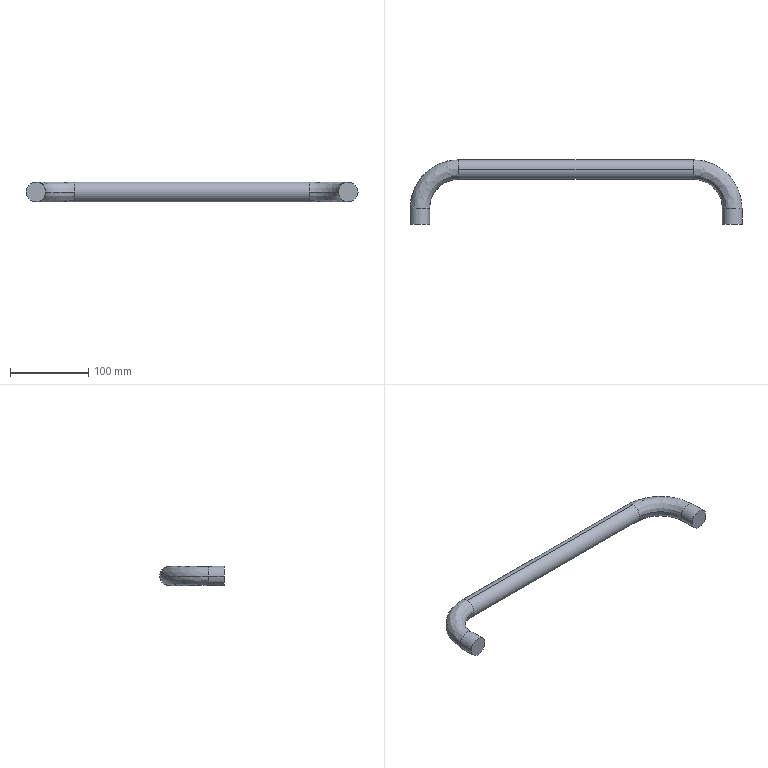Part | STEP file | 921270223 | 1 solid | 12 faces | box 425 x 82.5 x 25 mm | volume 244003 mm3 | cylinder 6 | spline 4 | plane 2 | commonest cylinder face diameters 25 x6
STEP:
#1=CARTESIAN_POINT('',(350.,82.5,0.));
#2=VERTEX_POINT('',#1);
#3=CARTESIAN_POINT('',(350.,70.,-12.5));
#4=VERTEX_POINT('',#3);
#5=CARTESIAN_POINT('',(350.,70.,0.));
#6=DIRECTION('',(-1.,0.,0.));
#7=DIRECTION('',(0.,0.,1.));
#8=AXIS2_PLACEMENT_3D('',#5,#6,#7);
#9=CIRCLE('',#8,12.5);
#10=EDGE_CURVE('',#2,#4,#9,.T.);
#11=ORIENTED_EDGE('',*,*,#10,.T.);
#12=CARTESIAN_POINT('',(50.,70.,-12.5));
#13=VERTEX_POINT('',#12);
#14=CARTESIAN_POINT('',(350.,70.,-12.5));
#15=DIRECTION('',(-1.,0.,0.));
#16=VECTOR('',#15,1000.);
#17=LINE('',#14,#16);
#18=EDGE_CURVE('',#4,#13,#17,.T.);
#19=ORIENTED_EDGE('',*,*,#18,.T.);
#20=CARTESIAN_POINT('',(50.,82.5,0.));
#21=VERTEX_POINT('',#20);
#22=CARTESIAN_POINT('',(50.,70.,0.));
#23=DIRECTION('',(1.,0.,0.));
#24=DIRECTION('',(0.,0.,1.));
#25=AXIS2_PLACEMENT_3D('',#22,#23,#24);
#26=CIRCLE('',#25,12.5);
#27=EDGE_CURVE('',#13,#21,#26,.T.);
#28=ORIENTED_EDGE('',*,*,#27,.T.);
#29=CARTESIAN_POINT('',(50.,70.,12.5));
#30=VERTEX_POINT('',#29);
#31=CARTESIAN_POINT('',(50.,70.,0.));
#32=DIRECTION('',(1.,0.,0.));
#33=DIRECTION('',(0.,0.,1.));
#34=AXIS2_PLACEMENT_3D('',#31,#32,#33);
#35=CIRCLE('',#34,12.5);
#36=EDGE_CURVE('',#21,#30,#35,.T.);
#37=ORIENTED_EDGE('',*,*,#36,.T.);
#38=CARTESIAN_POINT('',(350.,70.,12.5));
#39=VERTEX_POINT('',#38);
#40=CARTESIAN_POINT('',(350.,70.,12.5));
#41=DIRECTION('',(-1.,0.,0.));
#42=VECTOR('',#41,1000.);
#43=LINE('',#40,#42);
#44=EDGE_CURVE('',#39,#30,#43,.T.);
#45=ORIENTED_EDGE('',*,*,#44,.F.);
#46=CARTESIAN_POINT('',(350.,70.,0.));
#47=DIRECTION('',(-1.,0.,0.));
#48=DIRECTION('',(0.,0.,1.));
#49=AXIS2_PLACEMENT_3D('',#46,#47,#48);
#50=CIRCLE('',#49,12.5);
#51=EDGE_CURVE('',#39,#2,#50,.T.);
#52=ORIENTED_EDGE('',*,*,#51,.T.);
#53=EDGE_LOOP('',(#11,#19,#28,#37,#45,#52));
#54=FACE_OUTER_BOUND('',#53,.T.);
#55=CARTESIAN_POINT('',(350.,70.,0.));
#56=DIRECTION('',(-1.,0.,0.));
#57=DIRECTION('',(0.,0.,1.));
#58=AXIS2_PLACEMENT_3D('',#55,#56,#57);
#59=CYLINDRICAL_SURFACE('',#58,12.5);
#60=ADVANCED_FACE('',(#54),#59,.T.);
#61=CARTESIAN_POINT('',(50.,57.5,0.));
#62=VERTEX_POINT('',#61);
#63=CARTESIAN_POINT('',(50.,70.,0.));
#64=DIRECTION('',(1.,0.,0.));
#65=DIRECTION('',(0.,0.,1.));
#66=AXIS2_PLACEMENT_3D('',#63,#64,#65);
#67=CIRCLE('',#66,12.5);
#68=EDGE_CURVE('',#62,#13,#67,.T.);
#69=ORIENTED_EDGE('',*,*,#68,.F.);
#70=CARTESIAN_POINT('',(12.5,20.,0.));
#71=VERTEX_POINT('',#70);
#72=CARTESIAN_POINT('',(50.,20.,0.));
#73=DIRECTION('',(0.,0.,1.));
#74=DIRECTION('',(1.,0.,0.));
#75=AXIS2_PLACEMENT_3D('',#72,#73,#74);
#76=CIRCLE('',#75,37.5);
#77=EDGE_CURVE('',#62,#71,#76,.T.);
#78=ORIENTED_EDGE('',*,*,#77,.T.);
#79=CARTESIAN_POINT('',(-12.5,20.,0.));
#80=VERTEX_POINT('',#79);
#81=CARTESIAN_POINT('',(0.,20.,0.));
#82=DIRECTION('',(0.,1.,0.));
#83=DIRECTION('',(-1.,0.,0.));
#84=AXIS2_PLACEMENT_3D('',#81,#82,#83);
#85=CIRCLE('',#84,12.5);
#86=EDGE_CURVE('',#71,#80,#85,.T.);
#87=ORIENTED_EDGE('',*,*,#86,.T.);
#88=CARTESIAN_POINT('',(50.,20.,0.));
#89=DIRECTION('',(0.,0.,1.));
#90=DIRECTION('',(1.,0.,0.));
#91=AXIS2_PLACEMENT_3D('',#88,#89,#90);
#92=CIRCLE('',#91,62.5);
#93=EDGE_CURVE('',#21,#80,#92,.T.);
#94=ORIENTED_EDGE('',*,*,#93,.F.);
#95=ORIENTED_EDGE('',*,*,#27,.F.);
#96=EDGE_LOOP('',(#69,#78,#87,#94,#95));
#97=FACE_OUTER_BOUND('',#96,.T.);
#98=CARTESIAN_POINT('',(50.,82.5,0.));
#99=CARTESIAN_POINT('',(13.388,82.5,0.));
#100=CARTESIAN_POINT('',(-12.5,56.612,0.));
#101=CARTESIAN_POINT('',(-12.5,20.,0.));
#102=CARTESIAN_POINT('',(50.,82.5,-25.));
#103=CARTESIAN_POINT('',(13.388,82.5,-25.));
#104=CARTESIAN_POINT('',(-12.5,56.612,-25.));
#105=CARTESIAN_POINT('',(-12.5,20.,-25.));
#106=CARTESIAN_POINT('',(50.,57.5,-25.));
#107=CARTESIAN_POINT('',(28.033,57.5,-25.));
#108=CARTESIAN_POINT('',(12.5,41.967,-25.));
#109=CARTESIAN_POINT('',(12.5,20.,-25.));
#110=CARTESIAN_POINT('',(50.,57.5,0.));
#111=CARTESIAN_POINT('',(28.033,57.5,0.));
#112=CARTESIAN_POINT('',(12.5,41.967,0.));
#113=CARTESIAN_POINT('',(12.5,20.,0.));
#114=(BOUNDED_SURFACE()B_SPLINE_SURFACE(3,3,((#98,#99,#100,#101),(#102,#103,#104,#105),(#106,#107,#108,#109),(#110,#111,#112,#113)),.UNSPECIFIED.,.F.,.F.,.F.)B_SPLINE_SURFACE_WITH_KNOTS((4,4),(4,4),(0.,1.),(0.,1.),.UNSPECIFIED.)GEOMETRIC_REPRESENTATION_ITEM()RATIONAL_B_SPLINE_SURFACE(((1.,0.8047,0.8047,1.),(0.3333,0.2682,0.2682,0.3333),(0.3333,0.2682,0.2682,0.3333),(1.,0.8047,0.8047,1.)))REPRESENTATION_ITEM('')SURFACE());
#115=ADVANCED_FACE('',(#97),#114,.T.);
#116=CARTESIAN_POINT('',(412.5,20.,0.));
#117=VERTEX_POINT('',#116);
#118=CARTESIAN_POINT('',(387.5,20.,0.));
#119=VERTEX_POINT('',#118);
#120=CARTESIAN_POINT('',(400.,20.,0.));
#121=DIRECTION('',(0.,1.,0.));
#122=DIRECTION('',(1.,0.,0.));
#123=AXIS2_PLACEMENT_3D('',#120,#121,#122);
#124=CIRCLE('',#123,12.5);
#125=EDGE_CURVE('',#117,#119,#124,.T.);
#126=ORIENTED_EDGE('',*,*,#125,.T.);
#127=CARTESIAN_POINT('',(350.,57.5,0.));
#128=VERTEX_POINT('',#127);
#129=CARTESIAN_POINT('',(350.,20.,0.));
#130=DIRECTION('',(0.,0.,1.));
#131=DIRECTION('',(1.,0.,0.));
#132=AXIS2_PLACEMENT_3D('',#129,#130,#131);
#133=CIRCLE('',#132,37.5);
#134=EDGE_CURVE('',#119,#128,#133,.T.);
#135=ORIENTED_EDGE('',*,*,#134,.T.);
#136=CARTESIAN_POINT('',(350.,70.,0.));
#137=DIRECTION('',(-1.,0.,0.));
#138=DIRECTION('',(0.,0.,1.));
#139=AXIS2_PLACEMENT_3D('',#136,#137,#138);
#140=CIRCLE('',#139,12.5);
#141=EDGE_CURVE('',#4,#128,#140,.T.);
#142=ORIENTED_EDGE('',*,*,#141,.F.);
#143=ORIENTED_EDGE('',*,*,#10,.F.);
#144=CARTESIAN_POINT('',(350.,20.,0.));
#145=DIRECTION('',(0.,0.,1.));
#146=DIRECTION('',(1.,0.,0.));
#147=AXIS2_PLACEMENT_3D('',#144,#145,#146);
#148=CIRCLE('',#147,62.5);
#149=EDGE_CURVE('',#117,#2,#148,.T.);
#150=ORIENTED_EDGE('',*,*,#149,.F.);
#151=EDGE_LOOP('',(#126,#135,#142,#143,#150));
#152=FACE_OUTER_BOUND('',#151,.T.);
#153=CARTESIAN_POINT('',(412.5,20.,0.));
#154=CARTESIAN_POINT('',(412.5,56.612,0.));
#155=CARTESIAN_POINT('',(386.612,82.5,0.));
#156=CARTESIAN_POINT('',(350.,82.5,0.));
#157=CARTESIAN_POINT('',(412.5,20.,-25.));
#158=CARTESIAN_POINT('',(412.5,56.612,-25.));
#159=CARTESIAN_POINT('',(386.612,82.5,-25.));
#160=CARTESIAN_POINT('',(350.,82.5,-25.));
#161=CARTESIAN_POINT('',(387.5,20.,-25.));
#162=CARTESIAN_POINT('',(387.5,41.967,-25.));
#163=CARTESIAN_POINT('',(371.967,57.5,-25.));
#164=CARTESIAN_POINT('',(350.,57.5,-25.));
#165=CARTESIAN_POINT('',(387.5,20.,0.));
#166=CARTESIAN_POINT('',(387.5,41.967,0.));
#167=CARTESIAN_POINT('',(371.967,57.5,0.));
#168=CARTESIAN_POINT('',(350.,57.5,0.));
#169=(BOUNDED_SURFACE()B_SPLINE_SURFACE(3,3,((#153,#154,#155,#156),(#157,#158,#159,#160),(#161,#162,#163,#164),(#165,#166,#167,#168)),.UNSPECIFIED.,.F.,.F.,.F.)B_SPLINE_SURFACE_WITH_KNOTS((4,4),(4,4),(0.,1.),(0.,1.),.UNSPECIFIED.)GEOMETRIC_REPRESENTATION_ITEM()RATIONAL_B_SPLINE_SURFACE(((1.,0.8047,0.8047,1.),(0.3333,0.2682,0.2682,0.3333),(0.3333,0.2682,0.2682,0.3333),(1.,0.8047,0.8047,1.)))REPRESENTATION_ITEM('')SURFACE());
#170=ADVANCED_FACE('',(#152),#169,.T.);
#171=CARTESIAN_POINT('',(0.,20.,0.));
#172=DIRECTION('',(0.,1.,0.));
#173=DIRECTION('',(-1.,0.,0.));
#174=AXIS2_PLACEMENT_3D('',#171,#172,#173);
#175=CIRCLE('',#174,12.5);
#176=EDGE_CURVE('',#80,#71,#175,.T.);
#177=ORIENTED_EDGE('',*,*,#176,.F.);
#178=CARTESIAN_POINT('',(-12.5,0.,0.));
#179=VERTEX_POINT('',#178);
#180=CARTESIAN_POINT('',(-12.5,20.,0.));
#181=DIRECTION('',(0.,-1.,0.));
#182=VECTOR('',#181,1000.);
#183=LINE('',#180,#182);
#184=EDGE_CURVE('',#80,#179,#183,.T.);
#185=ORIENTED_EDGE('',*,*,#184,.T.);
#186=CARTESIAN_POINT('',(12.5,0.,0.));
#187=VERTEX_POINT('',#186);
#188=CARTESIAN_POINT('',(0.,0.,0.));
#189=DIRECTION('',(0.,1.,0.));
#190=DIRECTION('',(1.,0.,0.));
#191=AXIS2_PLACEMENT_3D('',#188,#189,#190);
#192=CIRCLE('',#191,12.5);
#193=EDGE_CURVE('',#179,#187,#192,.T.);
#194=ORIENTED_EDGE('',*,*,#193,.T.);
#195=CARTESIAN_POINT('',(12.5,20.,0.));
#196=DIRECTION('',(0.,-1.,0.));
#197=VECTOR('',#196,1000.);
#198=LINE('',#195,#197);
#199=EDGE_CURVE('',#71,#187,#198,.T.);
#200=ORIENTED_EDGE('',*,*,#199,.F.);
#201=EDGE_LOOP('',(#177,#185,#194,#200));
#202=FACE_OUTER_BOUND('',#201,.T.);
#203=CARTESIAN_POINT('',(0.,20.,0.));
#204=DIRECTION('',(0.,-1.,0.));
#205=DIRECTION('',(1.,0.,0.));
#206=AXIS2_PLACEMENT_3D('',#203,#204,#205);
#207=CYLINDRICAL_SURFACE('',#206,12.5);
#208=ADVANCED_FACE('',(#202),#207,.T.);
#209=CARTESIAN_POINT('',(400.,20.,0.));
#210=DIRECTION('',(0.,1.,0.));
#211=DIRECTION('',(1.,0.,0.));
#212=AXIS2_PLACEMENT_3D('',#209,#210,#211);
#213=CIRCLE('',#212,12.5);
#214=EDGE_CURVE('',#119,#117,#213,.T.);
#215=ORIENTED_EDGE('',*,*,#214,.F.);
#216=CARTESIAN_POINT('',(387.5,0.,0.));
#217=VERTEX_POINT('',#216);
#218=CARTESIAN_POINT('',(387.5,20.,0.));
#219=DIRECTION('',(0.,-1.,0.));
#220=VECTOR('',#219,1000.);
#221=LINE('',#218,#220);
#222=EDGE_CURVE('',#119,#217,#221,.T.);
#223=ORIENTED_EDGE('',*,*,#222,.T.);
#224=CARTESIAN_POINT('',(412.5,0.,0.));
#225=VERTEX_POINT('',#224);
#226=CARTESIAN_POINT('',(400.,0.,0.));
#227=DIRECTION('',(0.,1.,0.));
#228=DIRECTION('',(1.,0.,0.));
#229=AXIS2_PLACEMENT_3D('',#226,#227,#228);
#230=CIRCLE('',#229,12.5);
#231=EDGE_CURVE('',#217,#225,#230,.T.);
#232=ORIENTED_EDGE('',*,*,#231,.T.);
#233=CARTESIAN_POINT('',(412.5,20.,0.));
#234=DIRECTION('',(0.,-1.,0.));
#235=VECTOR('',#234,1000.);
#236=LINE('',#233,#235);
#237=EDGE_CURVE('',#117,#225,#236,.T.);
#238=ORIENTED_EDGE('',*,*,#237,.F.);
#239=EDGE_LOOP('',(#215,#223,#232,#238));
#240=FACE_OUTER_BOUND('',#239,.T.);
#241=CARTESIAN_POINT('',(400.,20.,0.));
#242=DIRECTION('',(0.,-1.,0.));
#243=DIRECTION('',(1.,0.,0.));
#244=AXIS2_PLACEMENT_3D('',#241,#242,#243);
#245=CYLINDRICAL_SURFACE('',#244,12.5);
#246=ADVANCED_FACE('',(#240),#245,.T.);
#247=ORIENTED_EDGE('',*,*,#18,.F.);
#248=ORIENTED_EDGE('',*,*,#141,.T.);
#249=CARTESIAN_POINT('',(350.,70.,0.));
#250=DIRECTION('',(-1.,0.,0.));
#251=DIRECTION('',(0.,0.,1.));
#252=AXIS2_PLACEMENT_3D('',#249,#250,#251);
#253=CIRCLE('',#252,12.5);
#254=EDGE_CURVE('',#128,#39,#253,.T.);
#255=ORIENTED_EDGE('',*,*,#254,.T.);
#256=ORIENTED_EDGE('',*,*,#44,.T.);
#257=CARTESIAN_POINT('',(50.,70.,0.));
#258=DIRECTION('',(1.,0.,0.));
#259=DIRECTION('',(0.,0.,1.));
#260=AXIS2_PLACEMENT_3D('',#257,#258,#259);
#261=CIRCLE('',#260,12.5);
#262=EDGE_CURVE('',#30,#62,#261,.T.);
#263=ORIENTED_EDGE('',*,*,#262,.T.);
#264=ORIENTED_EDGE('',*,*,#68,.T.);
#265=EDGE_LOOP('',(#247,#248,#255,#256,#263,#264));
#266=FACE_OUTER_BOUND('',#265,.T.);
#267=CARTESIAN_POINT('',(350.,70.,0.));
#268=DIRECTION('',(-1.,0.,0.));
#269=DIRECTION('',(0.,0.,1.));
#270=AXIS2_PLACEMENT_3D('',#267,#268,#269);
#271=CYLINDRICAL_SURFACE('',#270,12.5);
#272=ADVANCED_FACE('',(#266),#271,.T.);
#273=ORIENTED_EDGE('',*,*,#77,.F.);
#274=ORIENTED_EDGE('',*,*,#262,.F.);
#275=ORIENTED_EDGE('',*,*,#36,.F.);
#276=ORIENTED_EDGE('',*,*,#93,.T.);
#277=ORIENTED_EDGE('',*,*,#176,.T.);
#278=EDGE_LOOP('',(#273,#274,#275,#276,#277));
#279=FACE_OUTER_BOUND('',#278,.T.);
#280=CARTESIAN_POINT('',(50.,57.5,0.));
#281=CARTESIAN_POINT('',(28.033,57.5,0.));
#282=CARTESIAN_POINT('',(12.5,41.967,0.));
#283=CARTESIAN_POINT('',(12.5,20.,0.));
#284=CARTESIAN_POINT('',(50.,57.5,25.));
#285=CARTESIAN_POINT('',(28.033,57.5,25.));
#286=CARTESIAN_POINT('',(12.5,41.967,25.));
#287=CARTESIAN_POINT('',(12.5,20.,25.));
#288=CARTESIAN_POINT('',(50.,82.5,25.));
#289=CARTESIAN_POINT('',(13.388,82.5,25.));
#290=CARTESIAN_POINT('',(-12.5,56.612,25.));
#291=CARTESIAN_POINT('',(-12.5,20.,25.));
#292=CARTESIAN_POINT('',(50.,82.5,0.));
#293=CARTESIAN_POINT('',(13.388,82.5,0.));
#294=CARTESIAN_POINT('',(-12.5,56.612,0.));
#295=CARTESIAN_POINT('',(-12.5,20.,0.));
#296=(BOUNDED_SURFACE()B_SPLINE_SURFACE(3,3,((#280,#281,#282,#283),(#284,#285,#286,#287),(#288,#289,#290,#291),(#292,#293,#294,#295)),.UNSPECIFIED.,.F.,.F.,.F.)B_SPLINE_SURFACE_WITH_KNOTS((4,4),(4,4),(0.,1.),(0.,1.),.UNSPECIFIED.)GEOMETRIC_REPRESENTATION_ITEM()RATIONAL_B_SPLINE_SURFACE(((1.,0.8047,0.8047,1.),(0.3333,0.2682,0.2682,0.3333),(0.3333,0.2682,0.2682,0.3333),(1.,0.8047,0.8047,1.)))REPRESENTATION_ITEM('')SURFACE());
#297=ADVANCED_FACE('',(#279),#296,.T.);
#298=ORIENTED_EDGE('',*,*,#134,.F.);
#299=ORIENTED_EDGE('',*,*,#214,.T.);
#300=ORIENTED_EDGE('',*,*,#149,.T.);
#301=ORIENTED_EDGE('',*,*,#51,.F.);
#302=ORIENTED_EDGE('',*,*,#254,.F.);
#303=EDGE_LOOP('',(#298,#299,#300,#301,#302));
#304=FACE_OUTER_BOUND('',#303,.T.);
#305=CARTESIAN_POINT('',(387.5,20.,0.));
#306=CARTESIAN_POINT('',(387.5,41.967,0.));
#307=CARTESIAN_POINT('',(371.967,57.5,0.));
#308=CARTESIAN_POINT('',(350.,57.5,0.));
#309=CARTESIAN_POINT('',(387.5,20.,25.));
#310=CARTESIAN_POINT('',(387.5,41.967,25.));
#311=CARTESIAN_POINT('',(371.967,57.5,25.));
#312=CARTESIAN_POINT('',(350.,57.5,25.));
#313=CARTESIAN_POINT('',(412.5,20.,25.));
#314=CARTESIAN_POINT('',(412.5,56.612,25.));
#315=CARTESIAN_POINT('',(386.612,82.5,25.));
#316=CARTESIAN_POINT('',(350.,82.5,25.));
#317=CARTESIAN_POINT('',(412.5,20.,0.));
#318=CARTESIAN_POINT('',(412.5,56.612,0.));
#319=CARTESIAN_POINT('',(386.612,82.5,0.));
#320=CARTESIAN_POINT('',(350.,82.5,0.));
#321=(BOUNDED_SURFACE()B_SPLINE_SURFACE(3,3,((#305,#306,#307,#308),(#309,#310,#311,#312),(#313,#314,#315,#316),(#317,#318,#319,#320)),.UNSPECIFIED.,.F.,.F.,.F.)B_SPLINE_SURFACE_WITH_KNOTS((4,4),(4,4),(0.,1.),(0.,1.),.UNSPECIFIED.)GEOMETRIC_REPRESENTATION_ITEM()RATIONAL_B_SPLINE_SURFACE(((1.,0.8047,0.8047,1.),(0.3333,0.2682,0.2682,0.3333),(0.3333,0.2682,0.2682,0.3333),(1.,0.8047,0.8047,1.)))REPRESENTATION_ITEM('')SURFACE());
#322=ADVANCED_FACE('',(#304),#321,.T.);
#323=ORIENTED_EDGE('',*,*,#184,.F.);
#324=ORIENTED_EDGE('',*,*,#86,.F.);
#325=ORIENTED_EDGE('',*,*,#199,.T.);
#326=CARTESIAN_POINT('',(0.,0.,0.));
#327=DIRECTION('',(0.,1.,0.));
#328=DIRECTION('',(1.,0.,0.));
#329=AXIS2_PLACEMENT_3D('',#326,#327,#328);
#330=CIRCLE('',#329,12.5);
#331=EDGE_CURVE('',#187,#179,#330,.T.);
#332=ORIENTED_EDGE('',*,*,#331,.T.);
#333=EDGE_LOOP('',(#323,#324,#325,#332));
#334=FACE_OUTER_BOUND('',#333,.T.);
#335=CARTESIAN_POINT('',(0.,20.,0.));
#336=DIRECTION('',(0.,-1.,0.));
#337=DIRECTION('',(1.,0.,0.));
#338=AXIS2_PLACEMENT_3D('',#335,#336,#337);
#339=CYLINDRICAL_SURFACE('',#338,12.5);
#340=ADVANCED_FACE('',(#334),#339,.T.);
#341=ORIENTED_EDGE('',*,*,#222,.F.);
#342=ORIENTED_EDGE('',*,*,#125,.F.);
#343=ORIENTED_EDGE('',*,*,#237,.T.);
#344=CARTESIAN_POINT('',(400.,0.,0.));
#345=DIRECTION('',(0.,1.,0.));
#346=DIRECTION('',(1.,0.,0.));
#347=AXIS2_PLACEMENT_3D('',#344,#345,#346);
#348=CIRCLE('',#347,12.5);
#349=EDGE_CURVE('',#225,#217,#348,.T.);
#350=ORIENTED_EDGE('',*,*,#349,.T.);
#351=EDGE_LOOP('',(#341,#342,#343,#350));
#352=FACE_OUTER_BOUND('',#351,.T.);
#353=CARTESIAN_POINT('',(400.,20.,0.));
#354=DIRECTION('',(0.,-1.,0.));
#355=DIRECTION('',(1.,0.,0.));
#356=AXIS2_PLACEMENT_3D('',#353,#354,#355);
#357=CYLINDRICAL_SURFACE('',#356,12.5);
#358=ADVANCED_FACE('',(#352),#357,.T.);
#359=ORIENTED_EDGE('',*,*,#331,.F.);
#360=ORIENTED_EDGE('',*,*,#193,.F.);
#361=EDGE_LOOP('',(#359,#360));
#362=FACE_OUTER_BOUND('',#361,.T.);
#363=CARTESIAN_POINT('',(0.,0.,0.));
#364=DIRECTION('',(0.,-1.,0.));
#365=DIRECTION('',(1.,0.,0.));
#366=AXIS2_PLACEMENT_3D('',#363,#364,#365);
#367=PLANE('',#366);
#368=ADVANCED_FACE('',(#362),#367,.T.);
#369=ORIENTED_EDGE('',*,*,#349,.F.);
#370=ORIENTED_EDGE('',*,*,#231,.F.);
#371=EDGE_LOOP('',(#369,#370));
#372=FACE_OUTER_BOUND('',#371,.T.);
#373=CARTESIAN_POINT('',(400.,0.,0.));
#374=DIRECTION('',(0.,1.,0.));
#375=DIRECTION('',(-1.,0.,0.));
#376=AXIS2_PLACEMENT_3D('',#373,#374,#375);
#377=PLANE('',#376);
#378=ADVANCED_FACE('',(#372),#377,.F.);
#379=CLOSED_SHELL('',(#60,#115,#170,#208,#246,#272,#297,#322,#340,#358,#368,#378));
#380=MANIFOLD_SOLID_BREP('',#379);
#381=CARTESIAN_POINT('',(0.,0.,0.));
#382=DIRECTION('',(0.,0.,1.));
#383=DIRECTION('',(1.,0.,0.));
#384=AXIS2_PLACEMENT_3D('',#381,#382,#383);
#385=(LENGTH_UNIT()NAMED_UNIT(*)SI_UNIT(.MILLI.,.METRE.));
#386=UNCERTAINTY_MEASURE_WITH_UNIT(LENGTH_MEASURE(0.00001),#385,'','');
#387=(NAMED_UNIT(*)PLANE_ANGLE_UNIT()SI_UNIT($,.RADIAN.));
#388=(NAMED_UNIT(*)SI_UNIT($,.STERADIAN.)SOLID_ANGLE_UNIT());
#389=(GEOMETRIC_REPRESENTATION_CONTEXT(3)GLOBAL_UNCERTAINTY_ASSIGNED_CONTEXT((#386))GLOBAL_UNIT_ASSIGNED_CONTEXT((#385,#387,#388))REPRESENTATION_CONTEXT('',''));
#390=ADVANCED_BREP_SHAPE_REPRESENTATION('',(#380,#384),#389);